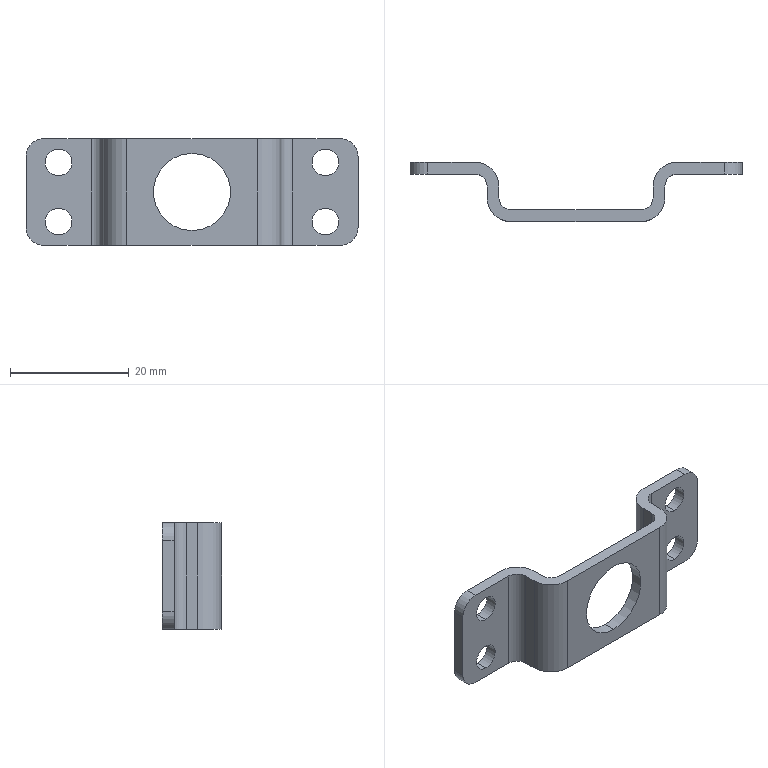Part | STEP file | Prox bracket-hub | 1 solid | 36 faces | box 56 x 10 x 18 mm | volume 1998 mm3 | cylinder 22 | plane 14 | commonest cylinder face diameters 4.5 x8 4 x4 6 x4 8 x4 13 x2